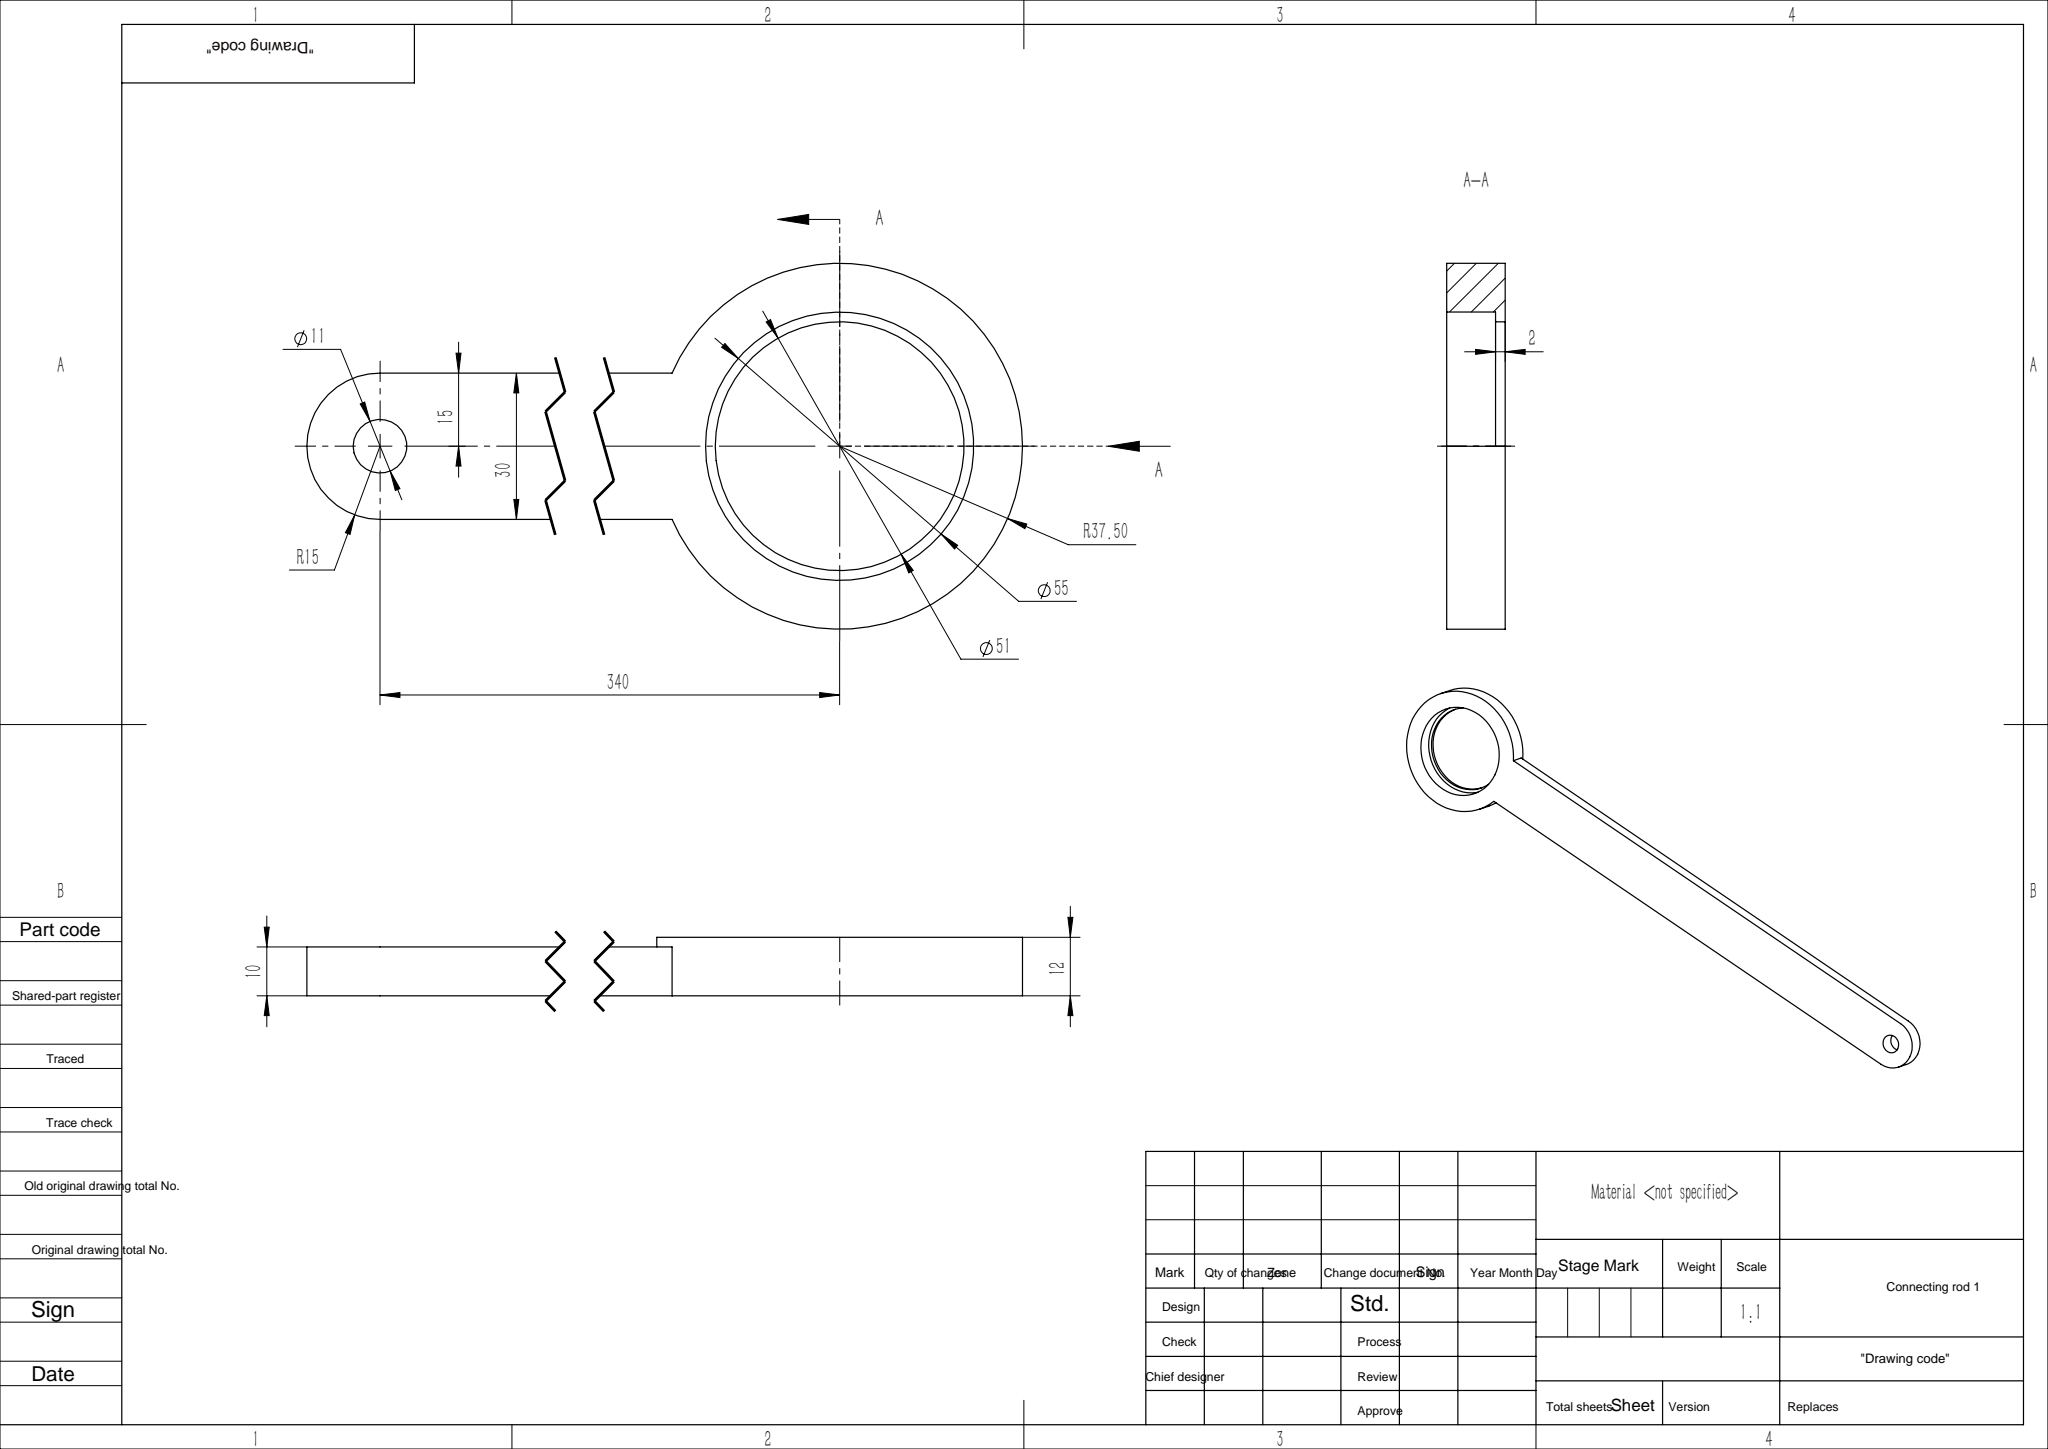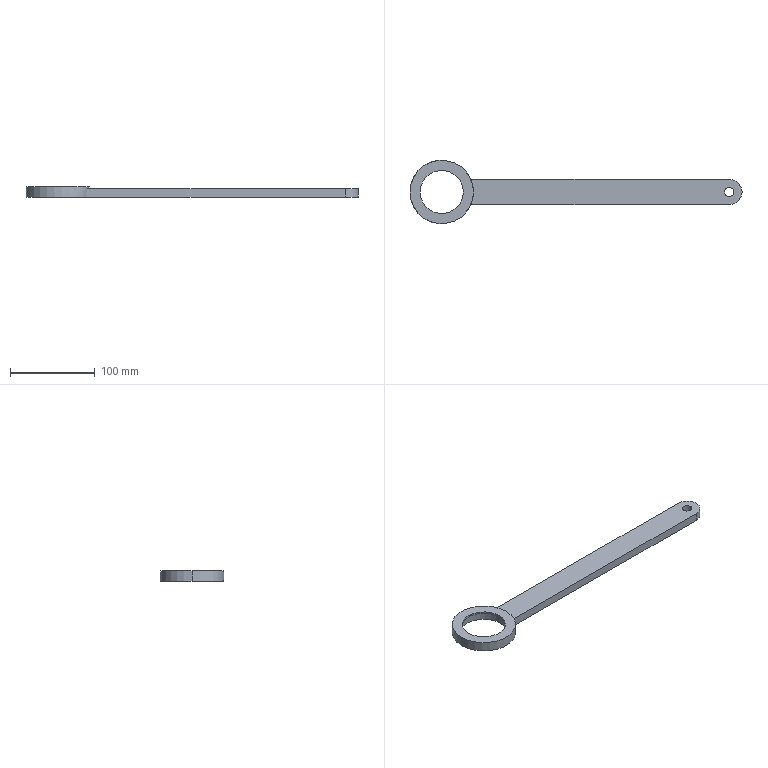Part | SolidWorks | features Extrusion 1, Fillet 1, ICE 1 | 1 solid | 16 faces | box 392.5 x 75 x 12 mm | volume 118812 mm3 | cylinder 10 | plane 6 | commonest cylinder face diameters 11 x2 30 x2 51 x2 55 x2 75 x2
STEP:
#1=CARTESIAN_POINT('',(-25.5,0.,12.));
#2=VERTEX_POINT('',#1);
#3=CARTESIAN_POINT('',(25.5,0.,12.));
#4=VERTEX_POINT('',#3);
#5=CARTESIAN_POINT('',(0.,0.,12.));
#6=DIRECTION('',(0.,0.,1.));
#7=DIRECTION('',(1.,0.,0.));
#8=AXIS2_PLACEMENT_3D('',#5,#6,#7);
#9=CIRCLE('',#8,25.5);
#10=EDGE_CURVE('',#2,#4,#9,.T.);
#11=ORIENTED_EDGE('',*,*,#10,.T.);
#12=CARTESIAN_POINT('',(25.5,0.,10.));
#13=VERTEX_POINT('',#12);
#14=CARTESIAN_POINT('',(25.5,0.,12.));
#15=DIRECTION('',(0.,0.,-1.));
#16=VECTOR('',#15,1000.);
#17=LINE('',#14,#16);
#18=EDGE_CURVE('',#4,#13,#17,.T.);
#19=ORIENTED_EDGE('',*,*,#18,.T.);
#20=CARTESIAN_POINT('',(-25.5,0.,10.));
#21=VERTEX_POINT('',#20);
#22=CARTESIAN_POINT('',(0.,0.,10.));
#23=DIRECTION('',(0.,0.,1.));
#24=DIRECTION('',(1.,0.,0.));
#25=AXIS2_PLACEMENT_3D('',#22,#23,#24);
#26=CIRCLE('',#25,25.5);
#27=EDGE_CURVE('',#21,#13,#26,.T.);
#28=ORIENTED_EDGE('',*,*,#27,.F.);
#29=CARTESIAN_POINT('',(-25.5,0.,12.));
#30=DIRECTION('',(0.,0.,-1.));
#31=VECTOR('',#30,1000.);
#32=LINE('',#29,#31);
#33=EDGE_CURVE('',#2,#21,#32,.T.);
#34=ORIENTED_EDGE('',*,*,#33,.F.);
#35=EDGE_LOOP('',(#11,#19,#28,#34));
#36=FACE_OUTER_BOUND('',#35,.T.);
#37=CARTESIAN_POINT('',(0.,0.,12.));
#38=DIRECTION('',(0.,0.,-1.));
#39=DIRECTION('',(-1.,0.,0.));
#40=AXIS2_PLACEMENT_3D('',#37,#38,#39);
#41=CYLINDRICAL_SURFACE('',#40,25.5);
#42=ADVANCED_FACE('',(#36),#41,.F.);
#43=CARTESIAN_POINT('',(-27.5,0.,10.));
#44=VERTEX_POINT('',#43);
#45=CARTESIAN_POINT('',(27.5,0.,10.));
#46=VERTEX_POINT('',#45);
#47=CARTESIAN_POINT('',(0.,0.,10.));
#48=DIRECTION('',(0.,0.,1.));
#49=DIRECTION('',(1.,0.,0.));
#50=AXIS2_PLACEMENT_3D('',#47,#48,#49);
#51=CIRCLE('',#50,27.5);
#52=EDGE_CURVE('',#44,#46,#51,.T.);
#53=ORIENTED_EDGE('',*,*,#52,.T.);
#54=CARTESIAN_POINT('',(27.5,0.,0.));
#55=VERTEX_POINT('',#54);
#56=CARTESIAN_POINT('',(27.5,0.,10.));
#57=DIRECTION('',(0.,0.,-1.));
#58=VECTOR('',#57,1000.);
#59=LINE('',#56,#58);
#60=EDGE_CURVE('',#46,#55,#59,.T.);
#61=ORIENTED_EDGE('',*,*,#60,.T.);
#62=CARTESIAN_POINT('',(-27.5,0.,0.));
#63=VERTEX_POINT('',#62);
#64=CARTESIAN_POINT('',(0.,0.,0.));
#65=DIRECTION('',(0.,0.,1.));
#66=DIRECTION('',(1.,0.,0.));
#67=AXIS2_PLACEMENT_3D('',#64,#65,#66);
#68=CIRCLE('',#67,27.5);
#69=EDGE_CURVE('',#63,#55,#68,.T.);
#70=ORIENTED_EDGE('',*,*,#69,.F.);
#71=CARTESIAN_POINT('',(-27.5,0.,10.));
#72=DIRECTION('',(0.,0.,-1.));
#73=VECTOR('',#72,1000.);
#74=LINE('',#71,#73);
#75=EDGE_CURVE('',#44,#63,#74,.T.);
#76=ORIENTED_EDGE('',*,*,#75,.F.);
#77=EDGE_LOOP('',(#53,#61,#70,#76));
#78=FACE_OUTER_BOUND('',#77,.T.);
#79=CARTESIAN_POINT('',(0.,0.,10.));
#80=DIRECTION('',(0.,0.,-1.));
#81=DIRECTION('',(-1.,0.,0.));
#82=AXIS2_PLACEMENT_3D('',#79,#80,#81);
#83=CYLINDRICAL_SURFACE('',#82,27.5);
#84=ADVANCED_FACE('',(#78),#83,.F.);
#85=CARTESIAN_POINT('',(334.5,0.,10.));
#86=VERTEX_POINT('',#85);
#87=CARTESIAN_POINT('',(345.5,0.,10.));
#88=VERTEX_POINT('',#87);
#89=CARTESIAN_POINT('',(340.,0.,10.));
#90=DIRECTION('',(0.,0.,1.));
#91=DIRECTION('',(1.,0.,0.));
#92=AXIS2_PLACEMENT_3D('',#89,#90,#91);
#93=CIRCLE('',#92,5.5);
#94=EDGE_CURVE('',#86,#88,#93,.T.);
#95=ORIENTED_EDGE('',*,*,#94,.T.);
#96=CARTESIAN_POINT('',(345.5,0.,0.));
#97=VERTEX_POINT('',#96);
#98=CARTESIAN_POINT('',(345.5,0.,10.));
#99=DIRECTION('',(0.,0.,-1.));
#100=VECTOR('',#99,1000.);
#101=LINE('',#98,#100);
#102=EDGE_CURVE('',#88,#97,#101,.T.);
#103=ORIENTED_EDGE('',*,*,#102,.T.);
#104=CARTESIAN_POINT('',(334.5,0.,0.));
#105=VERTEX_POINT('',#104);
#106=CARTESIAN_POINT('',(340.,0.,0.));
#107=DIRECTION('',(0.,0.,1.));
#108=DIRECTION('',(1.,0.,0.));
#109=AXIS2_PLACEMENT_3D('',#106,#107,#108);
#110=CIRCLE('',#109,5.5);
#111=EDGE_CURVE('',#105,#97,#110,.T.);
#112=ORIENTED_EDGE('',*,*,#111,.F.);
#113=CARTESIAN_POINT('',(334.5,0.,10.));
#114=DIRECTION('',(0.,0.,-1.));
#115=VECTOR('',#114,1000.);
#116=LINE('',#113,#115);
#117=EDGE_CURVE('',#86,#105,#116,.T.);
#118=ORIENTED_EDGE('',*,*,#117,.F.);
#119=EDGE_LOOP('',(#95,#103,#112,#118));
#120=FACE_OUTER_BOUND('',#119,.T.);
#121=CARTESIAN_POINT('',(340.,0.,10.));
#122=DIRECTION('',(0.,0.,-1.));
#123=DIRECTION('',(-1.,0.,0.));
#124=AXIS2_PLACEMENT_3D('',#121,#122,#123);
#125=CYLINDRICAL_SURFACE('',#124,5.5);
#126=ADVANCED_FACE('',(#120),#125,.F.);
#127=CARTESIAN_POINT('',(37.5,0.,12.));
#128=VERTEX_POINT('',#127);
#129=CARTESIAN_POINT('',(-37.5,0.,12.));
#130=VERTEX_POINT('',#129);
#131=CARTESIAN_POINT('',(0.,0.,12.));
#132=DIRECTION('',(0.,0.,1.));
#133=DIRECTION('',(1.,0.,0.));
#134=AXIS2_PLACEMENT_3D('',#131,#132,#133);
#135=CIRCLE('',#134,37.5);
#136=EDGE_CURVE('',#128,#130,#135,.T.);
#137=ORIENTED_EDGE('',*,*,#136,.F.);
#138=CARTESIAN_POINT('',(37.5,0.,10.));
#139=VERTEX_POINT('',#138);
#140=CARTESIAN_POINT('',(37.5,0.,10.));
#141=DIRECTION('',(0.,0.,-1.));
#142=VECTOR('',#141,1000.);
#143=LINE('',#140,#142);
#144=EDGE_CURVE('',#128,#139,#143,.T.);
#145=ORIENTED_EDGE('',*,*,#144,.T.);
#146=CARTESIAN_POINT('',(34.369,15.,10.));
#147=VERTEX_POINT('',#146);
#148=CARTESIAN_POINT('',(0.,0.,10.));
#149=DIRECTION('',(0.,0.,1.));
#150=DIRECTION('',(1.,0.,0.));
#151=AXIS2_PLACEMENT_3D('',#148,#149,#150);
#152=CIRCLE('',#151,37.5);
#153=EDGE_CURVE('',#139,#147,#152,.T.);
#154=ORIENTED_EDGE('',*,*,#153,.T.);
#155=CARTESIAN_POINT('',(34.369,15.,0.));
#156=VERTEX_POINT('',#155);
#157=CARTESIAN_POINT('',(34.369,15.,10.));
#158=DIRECTION('',(0.,0.,-1.));
#159=VECTOR('',#158,1000.);
#160=LINE('',#157,#159);
#161=EDGE_CURVE('',#147,#156,#160,.T.);
#162=ORIENTED_EDGE('',*,*,#161,.T.);
#163=CARTESIAN_POINT('',(-37.5,0.,0.));
#164=VERTEX_POINT('',#163);
#165=CARTESIAN_POINT('',(0.,0.,0.));
#166=DIRECTION('',(0.,0.,1.));
#167=DIRECTION('',(1.,0.,0.));
#168=AXIS2_PLACEMENT_3D('',#165,#166,#167);
#169=CIRCLE('',#168,37.5);
#170=EDGE_CURVE('',#156,#164,#169,.T.);
#171=ORIENTED_EDGE('',*,*,#170,.T.);
#172=CARTESIAN_POINT('',(-37.5,0.,10.));
#173=DIRECTION('',(0.,0.,-1.));
#174=VECTOR('',#173,1000.);
#175=LINE('',#172,#174);
#176=EDGE_CURVE('',#130,#164,#175,.T.);
#177=ORIENTED_EDGE('',*,*,#176,.F.);
#178=EDGE_LOOP('',(#137,#145,#154,#162,#171,#177));
#179=FACE_OUTER_BOUND('',#178,.T.);
#180=CARTESIAN_POINT('',(0.,0.,10.));
#181=DIRECTION('',(0.,0.,-1.));
#182=DIRECTION('',(-1.,0.,0.));
#183=AXIS2_PLACEMENT_3D('',#180,#181,#182);
#184=CYLINDRICAL_SURFACE('',#183,37.5);
#185=ADVANCED_FACE('',(#179),#184,.T.);
#186=CARTESIAN_POINT('',(34.369,-15.,10.));
#187=VERTEX_POINT('',#186);
#188=CARTESIAN_POINT('',(340.,-15.,10.));
#189=VERTEX_POINT('',#188);
#190=CARTESIAN_POINT('',(34.369,-15.,10.));
#191=DIRECTION('',(1.,0.,0.));
#192=VECTOR('',#191,1000.);
#193=LINE('',#190,#192);
#194=EDGE_CURVE('',#187,#189,#193,.T.);
#195=ORIENTED_EDGE('',*,*,#194,.T.);
#196=CARTESIAN_POINT('',(355.,0.,10.));
#197=VERTEX_POINT('',#196);
#198=CARTESIAN_POINT('',(340.,0.,10.));
#199=DIRECTION('',(0.,0.,1.));
#200=DIRECTION('',(1.,0.,0.));
#201=AXIS2_PLACEMENT_3D('',#198,#199,#200);
#202=CIRCLE('',#201,15.);
#203=EDGE_CURVE('',#189,#197,#202,.T.);
#204=ORIENTED_EDGE('',*,*,#203,.T.);
#205=CARTESIAN_POINT('',(340.,15.,10.));
#206=VERTEX_POINT('',#205);
#207=CARTESIAN_POINT('',(340.,0.,10.));
#208=DIRECTION('',(0.,0.,1.));
#209=DIRECTION('',(1.,0.,0.));
#210=AXIS2_PLACEMENT_3D('',#207,#208,#209);
#211=CIRCLE('',#210,15.);
#212=EDGE_CURVE('',#197,#206,#211,.T.);
#213=ORIENTED_EDGE('',*,*,#212,.T.);
#214=CARTESIAN_POINT('',(34.369,15.,10.));
#215=DIRECTION('',(-1.,0.,0.));
#216=VECTOR('',#215,1000.);
#217=LINE('',#214,#216);
#218=EDGE_CURVE('',#206,#147,#217,.T.);
#219=ORIENTED_EDGE('',*,*,#218,.T.);
#220=ORIENTED_EDGE('',*,*,#153,.F.);
#221=CARTESIAN_POINT('',(0.,0.,10.));
#222=DIRECTION('',(0.,0.,1.));
#223=DIRECTION('',(1.,0.,0.));
#224=AXIS2_PLACEMENT_3D('',#221,#222,#223);
#225=CIRCLE('',#224,37.5);
#226=EDGE_CURVE('',#187,#139,#225,.T.);
#227=ORIENTED_EDGE('',*,*,#226,.F.);
#228=EDGE_LOOP('',(#195,#204,#213,#219,#220,#227));
#229=FACE_OUTER_BOUND('',#228,.T.);
#230=ORIENTED_EDGE('',*,*,#94,.F.);
#231=CARTESIAN_POINT('',(340.,0.,10.));
#232=DIRECTION('',(0.,0.,1.));
#233=DIRECTION('',(1.,0.,0.));
#234=AXIS2_PLACEMENT_3D('',#231,#232,#233);
#235=CIRCLE('',#234,5.5);
#236=EDGE_CURVE('',#88,#86,#235,.T.);
#237=ORIENTED_EDGE('',*,*,#236,.F.);
#238=EDGE_LOOP('',(#230,#237));
#239=FACE_BOUND('',#238,.T.);
#240=CARTESIAN_POINT('',(0.,0.,10.));
#241=DIRECTION('',(0.,0.,1.));
#242=DIRECTION('',(1.,0.,0.));
#243=AXIS2_PLACEMENT_3D('',#240,#241,#242);
#244=PLANE('',#243);
#245=ADVANCED_FACE('',(#229,#239),#244,.T.);
#246=ORIENTED_EDGE('',*,*,#111,.T.);
#247=CARTESIAN_POINT('',(340.,0.,0.));
#248=DIRECTION('',(0.,0.,1.));
#249=DIRECTION('',(1.,0.,0.));
#250=AXIS2_PLACEMENT_3D('',#247,#248,#249);
#251=CIRCLE('',#250,5.5);
#252=EDGE_CURVE('',#97,#105,#251,.T.);
#253=ORIENTED_EDGE('',*,*,#252,.T.);
#254=EDGE_LOOP('',(#246,#253));
#255=FACE_BOUND('',#254,.T.);
#256=CARTESIAN_POINT('',(340.,15.,0.));
#257=VERTEX_POINT('',#256);
#258=CARTESIAN_POINT('',(355.,0.,0.));
#259=VERTEX_POINT('',#258);
#260=CARTESIAN_POINT('',(340.,0.,0.));
#261=DIRECTION('',(0.,0.,-1.));
#262=DIRECTION('',(1.,0.,0.));
#263=AXIS2_PLACEMENT_3D('',#260,#261,#262);
#264=CIRCLE('',#263,15.);
#265=EDGE_CURVE('',#257,#259,#264,.T.);
#266=ORIENTED_EDGE('',*,*,#265,.T.);
#267=CARTESIAN_POINT('',(340.,-15.,0.));
#268=VERTEX_POINT('',#267);
#269=CARTESIAN_POINT('',(340.,0.,0.));
#270=DIRECTION('',(0.,0.,-1.));
#271=DIRECTION('',(1.,0.,0.));
#272=AXIS2_PLACEMENT_3D('',#269,#270,#271);
#273=CIRCLE('',#272,15.);
#274=EDGE_CURVE('',#259,#268,#273,.T.);
#275=ORIENTED_EDGE('',*,*,#274,.T.);
#276=CARTESIAN_POINT('',(34.369,-15.,0.));
#277=VERTEX_POINT('',#276);
#278=CARTESIAN_POINT('',(34.369,-15.,0.));
#279=DIRECTION('',(1.,0.,0.));
#280=VECTOR('',#279,1000.);
#281=LINE('',#278,#280);
#282=EDGE_CURVE('',#277,#268,#281,.T.);
#283=ORIENTED_EDGE('',*,*,#282,.F.);
#284=CARTESIAN_POINT('',(0.,0.,0.));
#285=DIRECTION('',(0.,0.,1.));
#286=DIRECTION('',(1.,0.,0.));
#287=AXIS2_PLACEMENT_3D('',#284,#285,#286);
#288=CIRCLE('',#287,37.5);
#289=EDGE_CURVE('',#164,#277,#288,.T.);
#290=ORIENTED_EDGE('',*,*,#289,.F.);
#291=ORIENTED_EDGE('',*,*,#170,.F.);
#292=CARTESIAN_POINT('',(34.369,15.,0.));
#293=DIRECTION('',(-1.,0.,0.));
#294=VECTOR('',#293,1000.);
#295=LINE('',#292,#294);
#296=EDGE_CURVE('',#257,#156,#295,.T.);
#297=ORIENTED_EDGE('',*,*,#296,.F.);
#298=EDGE_LOOP('',(#266,#275,#283,#290,#291,#297));
#299=FACE_OUTER_BOUND('',#298,.T.);
#300=ORIENTED_EDGE('',*,*,#69,.T.);
#301=CARTESIAN_POINT('',(0.,0.,0.));
#302=DIRECTION('',(0.,0.,1.));
#303=DIRECTION('',(1.,0.,0.));
#304=AXIS2_PLACEMENT_3D('',#301,#302,#303);
#305=CIRCLE('',#304,27.5);
#306=EDGE_CURVE('',#55,#63,#305,.T.);
#307=ORIENTED_EDGE('',*,*,#306,.T.);
#308=EDGE_LOOP('',(#300,#307));
#309=FACE_BOUND('',#308,.T.);
#310=CARTESIAN_POINT('',(0.,0.,0.));
#311=DIRECTION('',(0.,0.,1.));
#312=DIRECTION('',(1.,0.,0.));
#313=AXIS2_PLACEMENT_3D('',#310,#311,#312);
#314=PLANE('',#313);
#315=ADVANCED_FACE('',(#255,#299,#309),#314,.F.);
#316=ORIENTED_EDGE('',*,*,#218,.F.);
#317=CARTESIAN_POINT('',(340.,15.,10.));
#318=DIRECTION('',(0.,0.,-1.));
#319=VECTOR('',#318,1000.);
#320=LINE('',#317,#319);
#321=EDGE_CURVE('',#206,#257,#320,.T.);
#322=ORIENTED_EDGE('',*,*,#321,.T.);
#323=ORIENTED_EDGE('',*,*,#296,.T.);
#324=ORIENTED_EDGE('',*,*,#161,.F.);
#325=EDGE_LOOP('',(#316,#322,#323,#324));
#326=FACE_OUTER_BOUND('',#325,.T.);
#327=CARTESIAN_POINT('',(34.369,15.,10.));
#328=DIRECTION('',(0.,-1.,0.));
#329=DIRECTION('',(0.,0.,-1.));
#330=AXIS2_PLACEMENT_3D('',#327,#328,#329);
#331=PLANE('',#330);
#332=ADVANCED_FACE('',(#326),#331,.F.);
#333=ORIENTED_EDGE('',*,*,#144,.F.);
#334=CARTESIAN_POINT('',(0.,0.,12.));
#335=DIRECTION('',(0.,0.,1.));
#336=DIRECTION('',(1.,0.,0.));
#337=AXIS2_PLACEMENT_3D('',#334,#335,#336);
#338=CIRCLE('',#337,37.5);
#339=EDGE_CURVE('',#130,#128,#338,.T.);
#340=ORIENTED_EDGE('',*,*,#339,.F.);
#341=ORIENTED_EDGE('',*,*,#176,.T.);
#342=ORIENTED_EDGE('',*,*,#289,.T.);
#343=CARTESIAN_POINT('',(34.369,-15.,10.));
#344=DIRECTION('',(0.,0.,-1.));
#345=VECTOR('',#344,1000.);
#346=LINE('',#343,#345);
#347=EDGE_CURVE('',#187,#277,#346,.T.);
#348=ORIENTED_EDGE('',*,*,#347,.F.);
#349=ORIENTED_EDGE('',*,*,#226,.T.);
#350=EDGE_LOOP('',(#333,#340,#341,#342,#348,#349));
#351=FACE_OUTER_BOUND('',#350,.T.);
#352=CARTESIAN_POINT('',(0.,0.,10.));
#353=DIRECTION('',(0.,0.,-1.));
#354=DIRECTION('',(-1.,0.,0.));
#355=AXIS2_PLACEMENT_3D('',#352,#353,#354);
#356=CYLINDRICAL_SURFACE('',#355,37.5);
#357=ADVANCED_FACE('',(#351),#356,.T.);
#358=ORIENTED_EDGE('',*,*,#282,.T.);
#359=CARTESIAN_POINT('',(340.,-15.,10.));
#360=DIRECTION('',(0.,0.,1.));
#361=VECTOR('',#360,1000.);
#362=LINE('',#359,#361);
#363=EDGE_CURVE('',#268,#189,#362,.T.);
#364=ORIENTED_EDGE('',*,*,#363,.T.);
#365=ORIENTED_EDGE('',*,*,#194,.F.);
#366=ORIENTED_EDGE('',*,*,#347,.T.);
#367=EDGE_LOOP('',(#358,#364,#365,#366));
#368=FACE_OUTER_BOUND('',#367,.T.);
#369=CARTESIAN_POINT('',(34.369,-15.,10.));
#370=DIRECTION('',(0.,1.,0.));
#371=DIRECTION('',(0.,0.,1.));
#372=AXIS2_PLACEMENT_3D('',#369,#370,#371);
#373=PLANE('',#372);
#374=ADVANCED_FACE('',(#368),#373,.F.);
#375=ORIENTED_EDGE('',*,*,#102,.F.);
#376=ORIENTED_EDGE('',*,*,#236,.T.);
#377=ORIENTED_EDGE('',*,*,#117,.T.);
#378=ORIENTED_EDGE('',*,*,#252,.F.);
#379=EDGE_LOOP('',(#375,#376,#377,#378));
#380=FACE_OUTER_BOUND('',#379,.T.);
#381=CARTESIAN_POINT('',(340.,0.,10.));
#382=DIRECTION('',(0.,0.,-1.));
#383=DIRECTION('',(-1.,0.,0.));
#384=AXIS2_PLACEMENT_3D('',#381,#382,#383);
#385=CYLINDRICAL_SURFACE('',#384,5.5);
#386=ADVANCED_FACE('',(#380),#385,.F.);
#387=ORIENTED_EDGE('',*,*,#60,.F.);
#388=CARTESIAN_POINT('',(0.,0.,10.));
#389=DIRECTION('',(0.,0.,1.));
#390=DIRECTION('',(1.,0.,0.));
#391=AXIS2_PLACEMENT_3D('',#388,#389,#390);
#392=CIRCLE('',#391,27.5);
#393=EDGE_CURVE('',#46,#44,#392,.T.);
#394=ORIENTED_EDGE('',*,*,#393,.T.);
#395=ORIENTED_EDGE('',*,*,#75,.T.);
#396=ORIENTED_EDGE('',*,*,#306,.F.);
#397=EDGE_LOOP('',(#387,#394,#395,#396));
#398=FACE_OUTER_BOUND('',#397,.T.);
#399=CARTESIAN_POINT('',(0.,0.,10.));
#400=DIRECTION('',(0.,0.,-1.));
#401=DIRECTION('',(-1.,0.,0.));
#402=AXIS2_PLACEMENT_3D('',#399,#400,#401);
#403=CYLINDRICAL_SURFACE('',#402,27.5);
#404=ADVANCED_FACE('',(#398),#403,.F.);
#405=ORIENTED_EDGE('',*,*,#339,.T.);
#406=ORIENTED_EDGE('',*,*,#136,.T.);
#407=EDGE_LOOP('',(#405,#406));
#408=FACE_OUTER_BOUND('',#407,.T.);
#409=ORIENTED_EDGE('',*,*,#10,.F.);
#410=CARTESIAN_POINT('',(0.,0.,12.));
#411=DIRECTION('',(0.,0.,1.));
#412=DIRECTION('',(1.,0.,0.));
#413=AXIS2_PLACEMENT_3D('',#410,#411,#412);
#414=CIRCLE('',#413,25.5);
#415=EDGE_CURVE('',#4,#2,#414,.T.);
#416=ORIENTED_EDGE('',*,*,#415,.F.);
#417=EDGE_LOOP('',(#409,#416));
#418=FACE_BOUND('',#417,.T.);
#419=CARTESIAN_POINT('',(0.,0.,12.));
#420=DIRECTION('',(0.,0.,1.));
#421=DIRECTION('',(1.,0.,0.));
#422=AXIS2_PLACEMENT_3D('',#419,#420,#421);
#423=PLANE('',#422);
#424=ADVANCED_FACE('',(#408,#418),#423,.T.);
#425=ORIENTED_EDGE('',*,*,#52,.F.);
#426=ORIENTED_EDGE('',*,*,#393,.F.);
#427=EDGE_LOOP('',(#425,#426));
#428=FACE_OUTER_BOUND('',#427,.T.);
#429=ORIENTED_EDGE('',*,*,#27,.T.);
#430=CARTESIAN_POINT('',(0.,0.,10.));
#431=DIRECTION('',(0.,0.,1.));
#432=DIRECTION('',(1.,0.,0.));
#433=AXIS2_PLACEMENT_3D('',#430,#431,#432);
#434=CIRCLE('',#433,25.5);
#435=EDGE_CURVE('',#13,#21,#434,.T.);
#436=ORIENTED_EDGE('',*,*,#435,.T.);
#437=EDGE_LOOP('',(#429,#436));
#438=FACE_BOUND('',#437,.T.);
#439=CARTESIAN_POINT('',(0.,0.,10.));
#440=DIRECTION('',(0.,0.,1.));
#441=DIRECTION('',(1.,0.,0.));
#442=AXIS2_PLACEMENT_3D('',#439,#440,#441);
#443=PLANE('',#442);
#444=ADVANCED_FACE('',(#428,#438),#443,.F.);
#445=ORIENTED_EDGE('',*,*,#18,.F.);
#446=ORIENTED_EDGE('',*,*,#415,.T.);
#447=ORIENTED_EDGE('',*,*,#33,.T.);
#448=ORIENTED_EDGE('',*,*,#435,.F.);
#449=EDGE_LOOP('',(#445,#446,#447,#448));
#450=FACE_OUTER_BOUND('',#449,.T.);
#451=CARTESIAN_POINT('',(0.,0.,12.));
#452=DIRECTION('',(0.,0.,-1.));
#453=DIRECTION('',(-1.,0.,0.));
#454=AXIS2_PLACEMENT_3D('',#451,#452,#453);
#455=CYLINDRICAL_SURFACE('',#454,25.5);
#456=ADVANCED_FACE('',(#450),#455,.F.);
#457=ORIENTED_EDGE('',*,*,#321,.F.);
#458=ORIENTED_EDGE('',*,*,#212,.F.);
#459=CARTESIAN_POINT('',(355.,0.,10.));
#460=DIRECTION('',(0.,0.,1.));
#461=VECTOR('',#460,1000.);
#462=LINE('',#459,#461);
#463=EDGE_CURVE('',#259,#197,#462,.T.);
#464=ORIENTED_EDGE('',*,*,#463,.F.);
#465=ORIENTED_EDGE('',*,*,#265,.F.);
#466=EDGE_LOOP('',(#457,#458,#464,#465));
#467=FACE_OUTER_BOUND('',#466,.T.);
#468=CARTESIAN_POINT('',(340.,0.,10.));
#469=DIRECTION('',(0.,0.,-1.));
#470=DIRECTION('',(-1.,0.,0.));
#471=AXIS2_PLACEMENT_3D('',#468,#469,#470);
#472=CYLINDRICAL_SURFACE('',#471,15.);
#473=ADVANCED_FACE('',(#467),#472,.T.);
#474=ORIENTED_EDGE('',*,*,#203,.F.);
#475=ORIENTED_EDGE('',*,*,#363,.F.);
#476=ORIENTED_EDGE('',*,*,#274,.F.);
#477=ORIENTED_EDGE('',*,*,#463,.T.);
#478=EDGE_LOOP('',(#474,#475,#476,#477));
#479=FACE_OUTER_BOUND('',#478,.T.);
#480=CARTESIAN_POINT('',(340.,0.,10.));
#481=DIRECTION('',(0.,0.,-1.));
#482=DIRECTION('',(-1.,0.,0.));
#483=AXIS2_PLACEMENT_3D('',#480,#481,#482);
#484=CYLINDRICAL_SURFACE('',#483,15.);
#485=ADVANCED_FACE('',(#479),#484,.T.);
#486=CLOSED_SHELL('',(#42,#84,#126,#185,#245,#315,#332,#357,#374,#386,#404,#424,#444,#456,#473,#485));
#487=MANIFOLD_SOLID_BREP('',#486);
#488=CARTESIAN_POINT('',(0.,0.,0.));
#489=DIRECTION('',(0.,0.,1.));
#490=DIRECTION('',(1.,0.,0.));
#491=AXIS2_PLACEMENT_3D('',#488,#489,#490);
#492=(LENGTH_UNIT()NAMED_UNIT(*)SI_UNIT(.MILLI.,.METRE.));
#493=UNCERTAINTY_MEASURE_WITH_UNIT(LENGTH_MEASURE(0.00001),#492,'','');
#494=(NAMED_UNIT(*)PLANE_ANGLE_UNIT()SI_UNIT($,.RADIAN.));
#495=(NAMED_UNIT(*)SI_UNIT($,.STERADIAN.)SOLID_ANGLE_UNIT());
#496=(GEOMETRIC_REPRESENTATION_CONTEXT(3)GLOBAL_UNCERTAINTY_ASSIGNED_CONTEXT((#493))GLOBAL_UNIT_ASSIGNED_CONTEXT((#492,#494,#495))REPRESENTATION_CONTEXT('',''));
#497=ADVANCED_BREP_SHAPE_REPRESENTATION('',(#487,#491),#496);